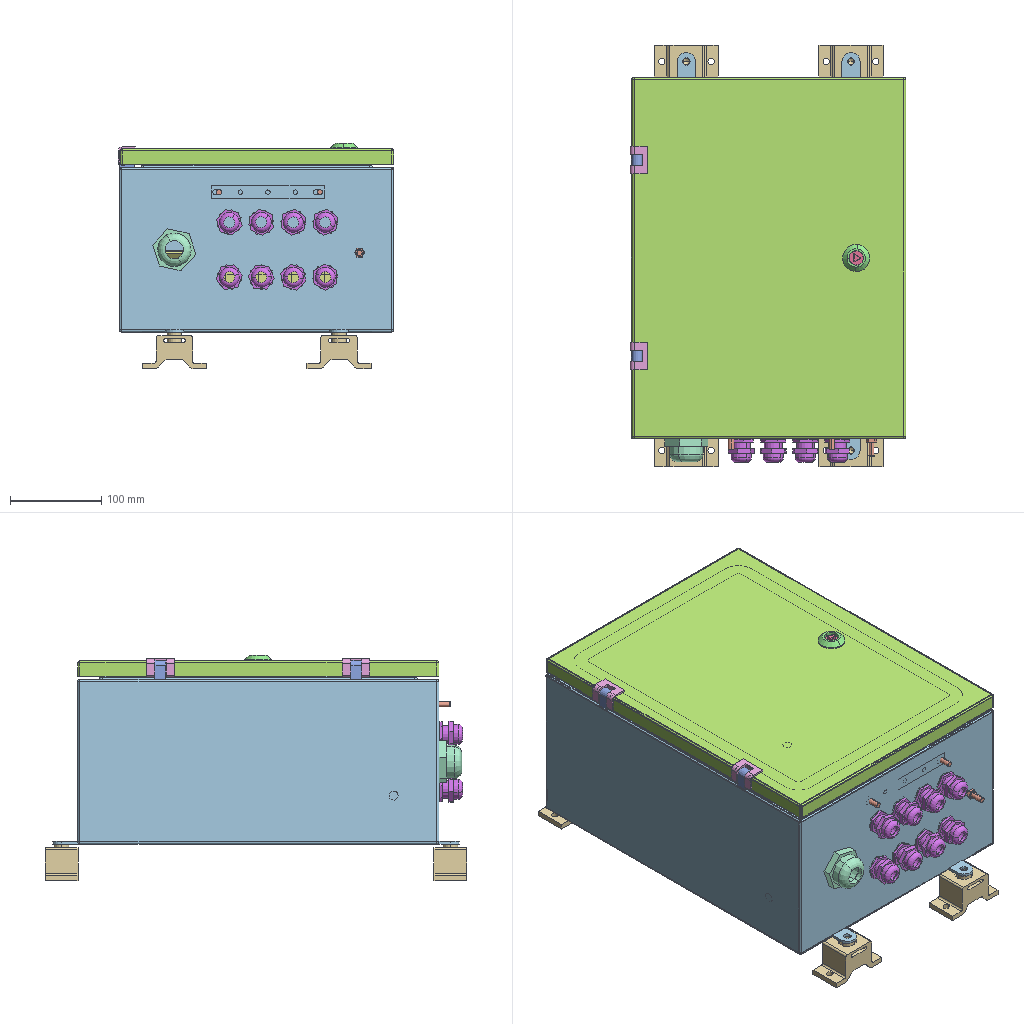Assembly | SolidWorks | 12 different items | 38 placed | box 302 x 461 x 246 mm
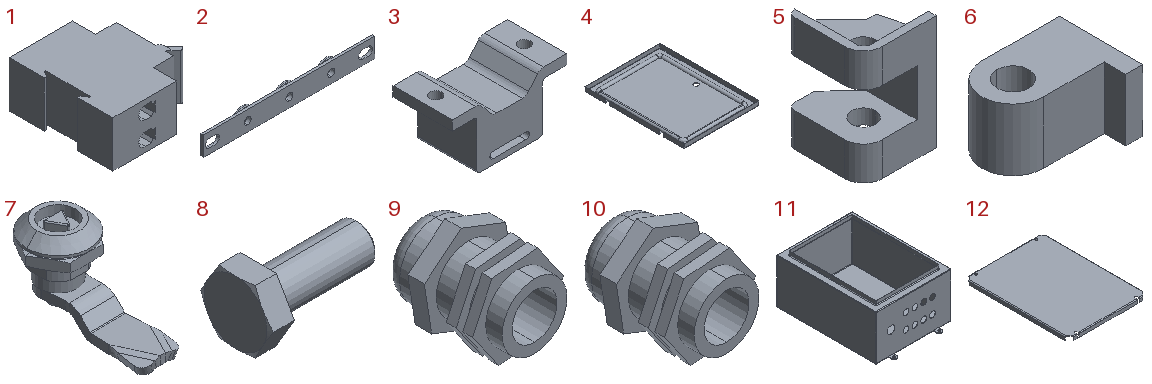Parts list (item | quantity | size | volume | features):
1 | x7 | 74.887 x 81 x 36 mm | 158863 mm3 | features ICE 7, ConnectionPoint 4, Chamfer 1, CombineBodies 1, Extrusion 1, Fillet 1, LPattern 1, MirrorPattern 1, PLine 1
2 | x1 | 123 x 4 x 15 mm | 4060 mm3 | features ICE 2, Extrusion 1
3 | x4 | 70 x 36 x 40.002 mm | 44732 mm3 | features Fillet 3, ICE 3, Extrusion 1, HoleWzd 1
4 | x1 | 299.3 x 395 x 17.2 mm | 268537 mm3 | features ICE 11, MoveFace 3, Fillet 2, BaseBody 1
5 | x2 | 19 x 20 x 30 mm | 3284 mm3 | features BaseBody 1
6 | x2 | 21 x 16.2 x 12 mm | 2422 mm3 | features BaseBody 1
7 | x1 | 31.177 x 64.298 x 36.976 mm | 13076 mm3 | features BaseBody 5
8 | x9 | 18.975 x 11.258 x 9.75 mm | 741.836 mm3 | features BaseBody 1, MoveFace 1, Scale 1
9 | x1 | 46.006 x 58.333 x 47.523 mm | 36742 mm3 | features ICE 5, Extrusion 1, Fillet 1, Scale 1, Shell 1
10 | x8 | 27.604 x 35 x 28.514 mm | 7936 mm3 | features ICE 5, Extrusion 1, Fillet 1, Shell 1
11 | x1 | 300 x 445.13 x 194.57 mm | 492765 mm3 | features ICE 3, Fillet 2, Extrusion 1, Shell 1
12 | x1 | 248 x 332 x 12.6 mm | 110968 mm3 | features BaseBody 1
Mates (type | each side: item.copy, entity, surface, feature):
Coincident | 12.1 face plane Input1 | 1.1 face plane Boss-Extrude1
Parallel | 11.1 face plane Shell1 | 1.1 face plane Split Line4
Coincident | 1.2 face plane LPattern2 | 1.3 face plane Split Line4
Coincident | 1.2 face plane Boss-Extrude1 | 1.3 face plane Boss-Extrude1 | 2 times
Coincident | 1.4 face plane Boss-Extrude1 | 1.5 face plane Boss-Extrude1 | 4 times
Coincident | 1.4 face plane LPattern2 | 1.5 face plane Split Line4
Coincident | 1.6 face plane Boss-Extrude1 | 1.7 face plane Boss-Extrude1 | 6 times
Coincident | 1.6 face plane LPattern2 | 1.7 face plane Split Line4
Coincident | 1.3 face plane LPattern2 | 1.4 face plane Split Line4
Coincident | 1.3 face plane Boss-Extrude1 | 1.4 face plane Boss-Extrude1 | 2 times
Coincident | 1.5 face plane LPattern2 | 1.6 face plane Split Line4
Coincident | 1.5 face plane Boss-Extrude1 | 1.6 face plane Boss-Extrude1 | 2 times
Coincident | 12.1 face plane Input1 | 1.7 face plane Boss-Extrude1
Coincident | 11.1 face plane Boss-Extrude1 | 8.1 face plane Input1
Coincident | 4.1 face plane Input1 | 8.2 face plane Input1
Coincident | 11.1 face plane Shell1 | 2.1 face plane Boss-Extrude1
Coincident | 11.1 face plane Shell1 | 8.3 face plane Input1
Concentric | 12.1 edge | 8.3 face cylinder Input1
Coincident | 11.1 face plane Shell1 | 8.4 face plane Input1
Concentric | 12.1 edge | 8.4 face cylinder Input1
Coincident | 11.1 face plane Shell1 | 8.5 face plane Input1
Concentric | 12.1 edge | 8.5 face cylinder Input1
Coincident | 11.1 face plane Shell1 | 8.6 face plane Input1
Concentric | 12.1 edge | 8.6 face cylinder Input1
Concentric | 2.1 face cylinder Boss-Extrude1 | 8.7 face cylinder Input1
Coincident | 2.1 face plane Boss-Extrude1 | 8.7 face plane Input1
Concentric | 2.1 face cylinder Boss-Extrude1 | 8.8 face cylinder Input1
Coincident | 2.1 face plane Boss-Extrude1 | 8.8 edge
Concentric | 11.1 edge | 9.1 face cylinder Boss-Extrude1
Coincident | 11.1 face plane Boss-Extrude1 | 9.1 face plane Boss-Extrude2
Concentric | 11.1 face cylinder Cut-Extrude1 | 10.1 face cylinder Boss-Extrude1
Coincident | 11.1 face plane Shell1 | 10.1 face plane Boss-Extrude5
Concentric | 11.1 edge | 10.2 face cylinder Boss-Extrude1
Coincident | 11.1 face plane Shell1 | 10.2 face plane Boss-Extrude5
Concentric | 11.1 edge | 10.3 face cylinder Boss-Extrude1
Coincident | 11.1 face plane Shell1 | 10.3 face plane Boss-Extrude5
Concentric | 11.1 edge | 10.4 face cylinder Boss-Extrude1
Coincident | 11.1 face plane Shell1 | 10.4 face plane Boss-Extrude5
Concentric | 11.1 edge | 10.5 face cylinder Boss-Extrude1
Coincident | 11.1 face plane Shell1 | 10.5 face plane Boss-Extrude5
Concentric | 11.1 face cylinder Cut-Extrude1 | 10.6 face cylinder Boss-Extrude1
Coincident | 11.1 face plane Shell1 | 10.6 face plane Boss-Extrude5
Concentric | 11.1 edge | 10.7 face cylinder Boss-Extrude1
Coincident | 11.1 face plane Shell1 | 10.7 face plane Boss-Extrude5
Concentric | 11.1 edge | 10.8 face cylinder Boss-Extrude1
Coincident | 11.1 face plane Shell1 | 10.8 face plane Boss-Extrude5
Coincident | 11.1 face plane Shell1 | 8.9 face plane Input1
Concentric | 11.1 face cylinder Boss-Extrude3 | 3.1 face cylinder M8 Tapped Hole1
Coincident | 11.1 face plane Boss-Extrude3 | 3.1 face plane Boss-Extrude2
Concentric | 11.1 face cylinder Boss-Extrude3 | 3.2 face cylinder M8 Tapped Hole1
Coincident | 11.1 face plane Boss-Extrude3 | 3.2 face plane Boss-Extrude2
Concentric | 11.1 face cylinder Boss-Extrude3 | 3.3 face cylinder M8 Tapped Hole1
Coincident | 11.1 face plane Boss-Extrude3 | 3.3 face plane Boss-Extrude2
Concentric | 11.1 face cylinder Boss-Extrude3 | 3.4 face cylinder M8 Tapped Hole1
Coincident | 11.1 face plane Boss-Extrude3 | 3.4 face plane Boss-Extrude2
Coincident | 3.3 face plane Boss-Extrude1 | 3.4 face plane Boss-Extrude1
Parallel | 3.1 face plane Boss-Extrude1 | 3.3 face plane Boss-Extrude1
Coincident | 3.1 face plane Boss-Extrude1 | 3.2 face plane Boss-Extrude1